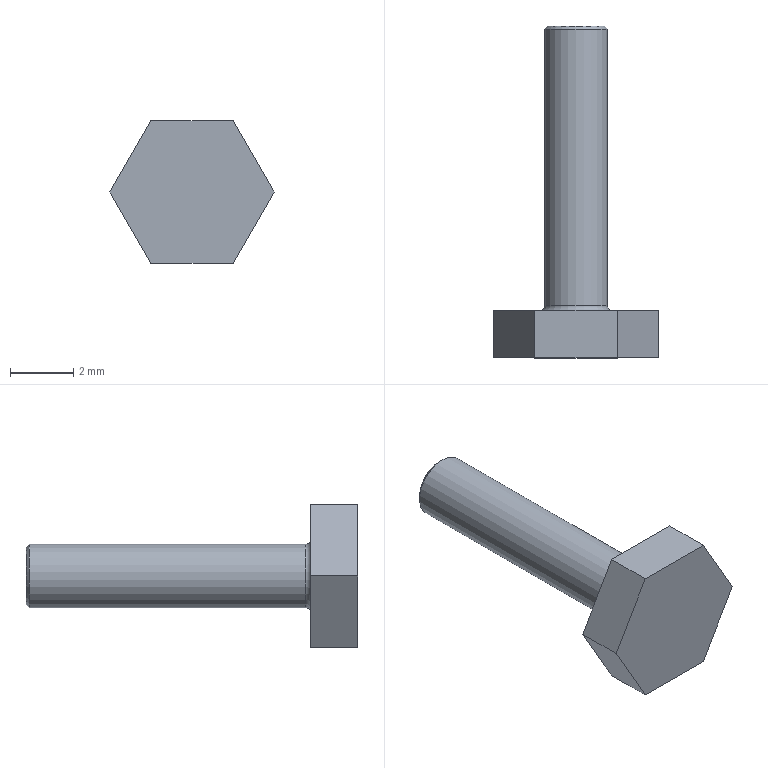Part | NX | features BREP 1 | 1 solid | 12 faces | box 5.196 x 10.5 x 4.5 mm | volume 54.581 mm3 | plane 9 | cylinder 1 | cone 1 | torus 1 | commonest cylinder face diameters 2 x1
STEP:
#1=CARTESIAN_POINT('',(1.299,0.,2.25));
#2=VERTEX_POINT('',#1);
#3=CARTESIAN_POINT('',(2.598,0.,0.));
#4=VERTEX_POINT('',#3);
#5=CARTESIAN_POINT('',(1.299,0.,2.25));
#6=DIRECTION('',(0.5,0.,-0.866));
#7=VECTOR('',#6,1000.);
#8=LINE('',#5,#7);
#9=EDGE_CURVE('',#2,#4,#8,.T.);
#10=ORIENTED_EDGE('',*,*,#9,.T.);
#11=CARTESIAN_POINT('',(2.598,1.5,0.));
#12=VERTEX_POINT('',#11);
#13=CARTESIAN_POINT('',(2.598,1.5,0.));
#14=DIRECTION('',(0.,-1.,0.));
#15=VECTOR('',#14,1000.);
#16=LINE('',#13,#15);
#17=EDGE_CURVE('',#12,#4,#16,.T.);
#18=ORIENTED_EDGE('',*,*,#17,.F.);
#19=CARTESIAN_POINT('',(1.299,1.5,2.25));
#20=VERTEX_POINT('',#19);
#21=CARTESIAN_POINT('',(1.299,1.5,2.25));
#22=DIRECTION('',(0.5,0.,-0.866));
#23=VECTOR('',#22,1000.);
#24=LINE('',#21,#23);
#25=EDGE_CURVE('',#20,#12,#24,.T.);
#26=ORIENTED_EDGE('',*,*,#25,.F.);
#27=CARTESIAN_POINT('',(1.299,1.5,2.25));
#28=DIRECTION('',(0.,-1.,0.));
#29=VECTOR('',#28,1000.);
#30=LINE('',#27,#29);
#31=EDGE_CURVE('',#20,#2,#30,.T.);
#32=ORIENTED_EDGE('',*,*,#31,.T.);
#33=EDGE_LOOP('',(#10,#18,#26,#32));
#34=FACE_BOUND('',#33,.T.);
#35=CARTESIAN_POINT('',(1.299,1.5,2.25));
#36=DIRECTION('',(-0.866,0.,-0.5));
#37=DIRECTION('',(0.5,0.,-0.866));
#38=AXIS2_PLACEMENT_3D('',#35,#36,#37);
#39=PLANE('',#38);
#40=ADVANCED_FACE('',(#34),#39,.F.);
#41=CARTESIAN_POINT('',(1.299,0.,-2.25));
#42=VERTEX_POINT('',#41);
#43=CARTESIAN_POINT('',(2.598,0.,0.));
#44=DIRECTION('',(-0.5,0.,-0.866));
#45=VECTOR('',#44,1000.);
#46=LINE('',#43,#45);
#47=EDGE_CURVE('',#4,#42,#46,.T.);
#48=ORIENTED_EDGE('',*,*,#47,.T.);
#49=CARTESIAN_POINT('',(1.299,1.5,-2.25));
#50=VERTEX_POINT('',#49);
#51=CARTESIAN_POINT('',(1.299,1.5,-2.25));
#52=DIRECTION('',(0.,-1.,0.));
#53=VECTOR('',#52,1000.);
#54=LINE('',#51,#53);
#55=EDGE_CURVE('',#50,#42,#54,.T.);
#56=ORIENTED_EDGE('',*,*,#55,.F.);
#57=CARTESIAN_POINT('',(2.598,1.5,0.));
#58=DIRECTION('',(-0.5,0.,-0.866));
#59=VECTOR('',#58,1000.);
#60=LINE('',#57,#59);
#61=EDGE_CURVE('',#12,#50,#60,.T.);
#62=ORIENTED_EDGE('',*,*,#61,.F.);
#63=ORIENTED_EDGE('',*,*,#17,.T.);
#64=EDGE_LOOP('',(#48,#56,#62,#63));
#65=FACE_BOUND('',#64,.T.);
#66=CARTESIAN_POINT('',(2.598,1.5,0.));
#67=DIRECTION('',(-0.866,0.,0.5));
#68=DIRECTION('',(-0.5,0.,-0.866));
#69=AXIS2_PLACEMENT_3D('',#66,#67,#68);
#70=PLANE('',#69);
#71=ADVANCED_FACE('',(#65),#70,.F.);
#72=CARTESIAN_POINT('',(-1.299,0.,-2.25));
#73=VERTEX_POINT('',#72);
#74=CARTESIAN_POINT('',(1.299,0.,-2.25));
#75=DIRECTION('',(-1.,0.,0.));
#76=VECTOR('',#75,1000.);
#77=LINE('',#74,#76);
#78=EDGE_CURVE('',#42,#73,#77,.T.);
#79=ORIENTED_EDGE('',*,*,#78,.T.);
#80=CARTESIAN_POINT('',(-1.299,1.5,-2.25));
#81=VERTEX_POINT('',#80);
#82=CARTESIAN_POINT('',(-1.299,1.5,-2.25));
#83=DIRECTION('',(0.,-1.,0.));
#84=VECTOR('',#83,1000.);
#85=LINE('',#82,#84);
#86=EDGE_CURVE('',#81,#73,#85,.T.);
#87=ORIENTED_EDGE('',*,*,#86,.F.);
#88=CARTESIAN_POINT('',(1.299,1.5,-2.25));
#89=DIRECTION('',(-1.,0.,0.));
#90=VECTOR('',#89,1000.);
#91=LINE('',#88,#90);
#92=EDGE_CURVE('',#50,#81,#91,.T.);
#93=ORIENTED_EDGE('',*,*,#92,.F.);
#94=ORIENTED_EDGE('',*,*,#55,.T.);
#95=EDGE_LOOP('',(#79,#87,#93,#94));
#96=FACE_BOUND('',#95,.T.);
#97=CARTESIAN_POINT('',(1.299,1.5,-2.25));
#98=DIRECTION('',(0.,0.,1.));
#99=DIRECTION('',(-1.,0.,0.));
#100=AXIS2_PLACEMENT_3D('',#97,#98,#99);
#101=PLANE('',#100);
#102=ADVANCED_FACE('',(#96),#101,.F.);
#103=CARTESIAN_POINT('',(-2.598,0.,0.));
#104=VERTEX_POINT('',#103);
#105=CARTESIAN_POINT('',(-1.299,0.,-2.25));
#106=DIRECTION('',(-0.5,0.,0.866));
#107=VECTOR('',#106,1000.);
#108=LINE('',#105,#107);
#109=EDGE_CURVE('',#73,#104,#108,.T.);
#110=ORIENTED_EDGE('',*,*,#109,.T.);
#111=CARTESIAN_POINT('',(-2.598,1.5,0.));
#112=VERTEX_POINT('',#111);
#113=CARTESIAN_POINT('',(-2.598,1.5,0.));
#114=DIRECTION('',(0.,-1.,0.));
#115=VECTOR('',#114,1000.);
#116=LINE('',#113,#115);
#117=EDGE_CURVE('',#112,#104,#116,.T.);
#118=ORIENTED_EDGE('',*,*,#117,.F.);
#119=CARTESIAN_POINT('',(-1.299,1.5,-2.25));
#120=DIRECTION('',(-0.5,0.,0.866));
#121=VECTOR('',#120,1000.);
#122=LINE('',#119,#121);
#123=EDGE_CURVE('',#81,#112,#122,.T.);
#124=ORIENTED_EDGE('',*,*,#123,.F.);
#125=ORIENTED_EDGE('',*,*,#86,.T.);
#126=EDGE_LOOP('',(#110,#118,#124,#125));
#127=FACE_BOUND('',#126,.T.);
#128=CARTESIAN_POINT('',(-1.299,1.5,-2.25));
#129=DIRECTION('',(0.866,0.,0.5));
#130=DIRECTION('',(-0.5,0.,0.866));
#131=AXIS2_PLACEMENT_3D('',#128,#129,#130);
#132=PLANE('',#131);
#133=ADVANCED_FACE('',(#127),#132,.F.);
#134=CARTESIAN_POINT('',(-1.299,0.,2.25));
#135=VERTEX_POINT('',#134);
#136=CARTESIAN_POINT('',(-2.598,0.,0.));
#137=DIRECTION('',(0.5,0.,0.866));
#138=VECTOR('',#137,1000.);
#139=LINE('',#136,#138);
#140=EDGE_CURVE('',#104,#135,#139,.T.);
#141=ORIENTED_EDGE('',*,*,#140,.T.);
#142=CARTESIAN_POINT('',(-1.299,1.5,2.25));
#143=VERTEX_POINT('',#142);
#144=CARTESIAN_POINT('',(-1.299,1.5,2.25));
#145=DIRECTION('',(0.,-1.,0.));
#146=VECTOR('',#145,1000.);
#147=LINE('',#144,#146);
#148=EDGE_CURVE('',#143,#135,#147,.T.);
#149=ORIENTED_EDGE('',*,*,#148,.F.);
#150=CARTESIAN_POINT('',(-2.598,1.5,0.));
#151=DIRECTION('',(0.5,0.,0.866));
#152=VECTOR('',#151,1000.);
#153=LINE('',#150,#152);
#154=EDGE_CURVE('',#112,#143,#153,.T.);
#155=ORIENTED_EDGE('',*,*,#154,.F.);
#156=ORIENTED_EDGE('',*,*,#117,.T.);
#157=EDGE_LOOP('',(#141,#149,#155,#156));
#158=FACE_BOUND('',#157,.T.);
#159=CARTESIAN_POINT('',(-2.598,1.5,0.));
#160=DIRECTION('',(0.866,0.,-0.5));
#161=DIRECTION('',(0.5,0.,0.866));
#162=AXIS2_PLACEMENT_3D('',#159,#160,#161);
#163=PLANE('',#162);
#164=ADVANCED_FACE('',(#158),#163,.F.);
#165=CARTESIAN_POINT('',(-1.299,0.,2.25));
#166=DIRECTION('',(1.,0.,0.));
#167=VECTOR('',#166,1000.);
#168=LINE('',#165,#167);
#169=EDGE_CURVE('',#135,#2,#168,.T.);
#170=ORIENTED_EDGE('',*,*,#169,.T.);
#171=ORIENTED_EDGE('',*,*,#31,.F.);
#172=CARTESIAN_POINT('',(-1.299,1.5,2.25));
#173=DIRECTION('',(1.,0.,0.));
#174=VECTOR('',#173,1000.);
#175=LINE('',#172,#174);
#176=EDGE_CURVE('',#143,#20,#175,.T.);
#177=ORIENTED_EDGE('',*,*,#176,.F.);
#178=ORIENTED_EDGE('',*,*,#148,.T.);
#179=EDGE_LOOP('',(#170,#171,#177,#178));
#180=FACE_BOUND('',#179,.T.);
#181=CARTESIAN_POINT('',(-1.299,1.5,2.25));
#182=DIRECTION('',(0.,0.,-1.));
#183=DIRECTION('',(1.,0.,0.));
#184=AXIS2_PLACEMENT_3D('',#181,#182,#183);
#185=PLANE('',#184);
#186=ADVANCED_FACE('',(#180),#185,.F.);
#187=CARTESIAN_POINT('',(0.,1.5,1.15));
#188=VERTEX_POINT('',#187);
#189=CARTESIAN_POINT('',(0.,1.5,0.));
#190=DIRECTION('',(0.,-1.,0.));
#191=DIRECTION('',(0.,0.,1.));
#192=AXIS2_PLACEMENT_3D('',#189,#190,#191);
#193=CIRCLE('',#192,1.15);
#194=EDGE_CURVE('',#188,#188,#193,.T.);
#195=ORIENTED_EDGE('',*,*,#194,.T.);
#196=EDGE_LOOP('',(#195));
#197=FACE_BOUND('',#196,.T.);
#198=ORIENTED_EDGE('',*,*,#25,.T.);
#199=ORIENTED_EDGE('',*,*,#61,.T.);
#200=ORIENTED_EDGE('',*,*,#92,.T.);
#201=ORIENTED_EDGE('',*,*,#123,.T.);
#202=ORIENTED_EDGE('',*,*,#154,.T.);
#203=ORIENTED_EDGE('',*,*,#176,.T.);
#204=EDGE_LOOP('',(#198,#199,#200,#201,#202,#203));
#205=FACE_BOUND('',#204,.T.);
#206=CARTESIAN_POINT('',(0.,1.5,0.));
#207=DIRECTION('',(0.,1.,0.));
#208=DIRECTION('',(0.,0.,-1.));
#209=AXIS2_PLACEMENT_3D('',#206,#207,#208);
#210=PLANE('',#209);
#211=ADVANCED_FACE('',(#197,#205),#210,.T.);
#212=ORIENTED_EDGE('',*,*,#9,.F.);
#213=ORIENTED_EDGE('',*,*,#169,.F.);
#214=ORIENTED_EDGE('',*,*,#140,.F.);
#215=ORIENTED_EDGE('',*,*,#109,.F.);
#216=ORIENTED_EDGE('',*,*,#78,.F.);
#217=ORIENTED_EDGE('',*,*,#47,.F.);
#218=EDGE_LOOP('',(#212,#213,#214,#215,#216,#217));
#219=FACE_BOUND('',#218,.T.);
#220=CARTESIAN_POINT('',(0.,0.,0.));
#221=DIRECTION('',(0.,1.,0.));
#222=DIRECTION('',(0.,0.,-1.));
#223=AXIS2_PLACEMENT_3D('',#220,#221,#222);
#224=PLANE('',#223);
#225=ADVANCED_FACE('',(#219),#224,.F.);
#226=CARTESIAN_POINT('',(0.,1.65,1.));
#227=VERTEX_POINT('',#226);
#228=CARTESIAN_POINT('',(0.,1.65,0.));
#229=DIRECTION('',(0.,1.,0.));
#230=DIRECTION('',(0.,0.,1.));
#231=AXIS2_PLACEMENT_3D('',#228,#229,#230);
#232=CIRCLE('',#231,1.);
#233=EDGE_CURVE('',#227,#227,#232,.T.);
#234=ORIENTED_EDGE('',*,*,#233,.T.);
#235=EDGE_LOOP('',(#234));
#236=FACE_BOUND('',#235,.T.);
#237=CARTESIAN_POINT('',(0.,10.4,1.));
#238=VERTEX_POINT('',#237);
#239=CARTESIAN_POINT('',(0.,10.4,0.));
#240=DIRECTION('',(0.,-1.,0.));
#241=DIRECTION('',(0.,0.,1.));
#242=AXIS2_PLACEMENT_3D('',#239,#240,#241);
#243=CIRCLE('',#242,1.);
#244=EDGE_CURVE('',#238,#238,#243,.T.);
#245=ORIENTED_EDGE('',*,*,#244,.T.);
#246=EDGE_LOOP('',(#245));
#247=FACE_BOUND('',#246,.T.);
#248=CARTESIAN_POINT('',(0.,10.5,0.));
#249=DIRECTION('',(0.,-1.,0.));
#250=DIRECTION('',(0.,0.,1.));
#251=AXIS2_PLACEMENT_3D('',#248,#249,#250);
#252=CYLINDRICAL_SURFACE('',#251,1.);
#253=ADVANCED_FACE('',(#236,#247),#252,.T.);
#254=CARTESIAN_POINT('',(0.,10.5,0.9));
#255=VERTEX_POINT('',#254);
#256=CARTESIAN_POINT('',(0.,10.5,0.));
#257=DIRECTION('',(0.,1.,0.));
#258=DIRECTION('',(0.,0.,1.));
#259=AXIS2_PLACEMENT_3D('',#256,#257,#258);
#260=CIRCLE('',#259,0.9);
#261=EDGE_CURVE('',#255,#255,#260,.T.);
#262=ORIENTED_EDGE('',*,*,#261,.T.);
#263=EDGE_LOOP('',(#262));
#264=FACE_BOUND('',#263,.T.);
#265=CARTESIAN_POINT('',(0.,10.5,0.));
#266=DIRECTION('',(0.,1.,0.));
#267=DIRECTION('',(0.,0.,-1.));
#268=AXIS2_PLACEMENT_3D('',#265,#266,#267);
#269=PLANE('',#268);
#270=ADVANCED_FACE('',(#264),#269,.T.);
#271=ORIENTED_EDGE('',*,*,#244,.F.);
#272=EDGE_LOOP('',(#271));
#273=FACE_BOUND('',#272,.T.);
#274=ORIENTED_EDGE('',*,*,#261,.F.);
#275=EDGE_LOOP('',(#274));
#276=FACE_BOUND('',#275,.T.);
#277=CARTESIAN_POINT('',(0.,10.5,0.));
#278=DIRECTION('',(0.,-1.,0.));
#279=DIRECTION('',(0.,0.,1.));
#280=AXIS2_PLACEMENT_3D('',#277,#278,#279);
#281=CONICAL_SURFACE('',#280,0.9,0.7854);
#282=ADVANCED_FACE('',(#273,#276),#281,.T.);
#283=ORIENTED_EDGE('',*,*,#194,.F.);
#284=EDGE_LOOP('',(#283));
#285=FACE_BOUND('',#284,.T.);
#286=ORIENTED_EDGE('',*,*,#233,.F.);
#287=EDGE_LOOP('',(#286));
#288=FACE_BOUND('',#287,.T.);
#289=CARTESIAN_POINT('',(0.,1.65,0.));
#290=DIRECTION('',(0.,1.,0.));
#291=DIRECTION('',(0.,0.,-1.));
#292=AXIS2_PLACEMENT_3D('',#289,#290,#291);
#293=TOROIDAL_SURFACE('',#292,1.15,0.15);
#294=ADVANCED_FACE('',(#285,#288),#293,.F.);
#295=CLOSED_SHELL('',(#40,#71,#102,#133,#164,#186,#211,#225,#253,#270,#282,#294));
#296=MANIFOLD_SOLID_BREP('',#295);
#297=(LENGTH_UNIT()NAMED_UNIT(*)SI_UNIT(.MILLI.,.METRE.));
#298=UNCERTAINTY_MEASURE_WITH_UNIT(LENGTH_MEASURE(0.00001),#297,'','');
#299=(NAMED_UNIT(*)PLANE_ANGLE_UNIT()SI_UNIT($,.RADIAN.));
#300=(NAMED_UNIT(*)SI_UNIT($,.STERADIAN.)SOLID_ANGLE_UNIT());
#301=(GEOMETRIC_REPRESENTATION_CONTEXT(3)GLOBAL_UNCERTAINTY_ASSIGNED_CONTEXT((#298))GLOBAL_UNIT_ASSIGNED_CONTEXT((#297,#299,#300))REPRESENTATION_CONTEXT('',''));
#302=ADVANCED_BREP_SHAPE_REPRESENTATION('',(#296),#301);